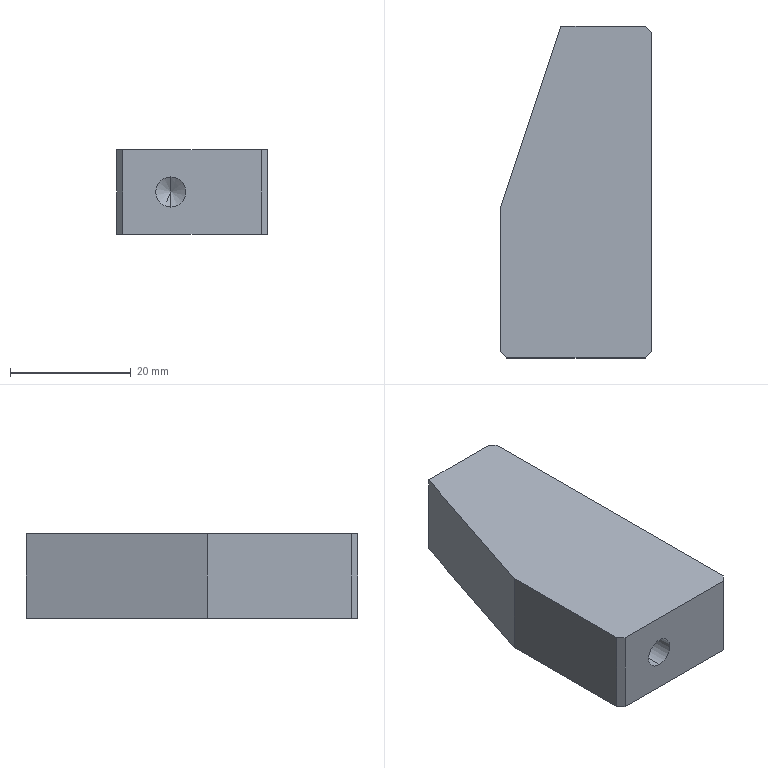Part | SolidWorks | features HoleWzd 2, Chamfer 1, Extrusion 1 | 1 solid | 22 faces | box 25 x 55 x 14 mm | volume 16216 mm3 | plane 10 | cylinder 6 | cone 6 | commonest cylinder face diameters 5 x6
STEP:
#1=CARTESIAN_POINT('',(-16.,15.,2.5));
#2=VERTEX_POINT('',#1);
#3=CARTESIAN_POINT('',(-16.,15.,-2.5));
#4=VERTEX_POINT('',#3);
#5=CARTESIAN_POINT('',(-16.,15.,0.));
#6=DIRECTION('',(0.,-1.,0.));
#7=DIRECTION('',(0.,0.,-1.));
#8=AXIS2_PLACEMENT_3D('',#5,#6,#7);
#9=CIRCLE('',#8,2.5);
#10=EDGE_CURVE('',#2,#4,#9,.T.);
#11=ORIENTED_EDGE('',*,*,#10,.F.);
#12=CARTESIAN_POINT('',(-16.,0.,2.5));
#13=VERTEX_POINT('',#12);
#14=CARTESIAN_POINT('',(-16.,0.,2.5));
#15=DIRECTION('',(0.,-1.,0.));
#16=VECTOR('',#15,1000.);
#17=LINE('',#14,#16);
#18=EDGE_CURVE('',#2,#13,#17,.T.);
#19=ORIENTED_EDGE('',*,*,#18,.T.);
#20=CARTESIAN_POINT('',(-16.,0.,-2.5));
#21=VERTEX_POINT('',#20);
#22=CARTESIAN_POINT('',(-16.,0.,0.));
#23=DIRECTION('',(0.,-1.,0.));
#24=DIRECTION('',(0.,0.,-1.));
#25=AXIS2_PLACEMENT_3D('',#22,#23,#24);
#26=CIRCLE('',#25,2.5);
#27=EDGE_CURVE('',#13,#21,#26,.T.);
#28=ORIENTED_EDGE('',*,*,#27,.T.);
#29=CARTESIAN_POINT('',(-16.,0.,-2.5));
#30=DIRECTION('',(0.,-1.,0.));
#31=VECTOR('',#30,1000.);
#32=LINE('',#29,#31);
#33=EDGE_CURVE('',#4,#21,#32,.T.);
#34=ORIENTED_EDGE('',*,*,#33,.F.);
#35=EDGE_LOOP('',(#11,#19,#28,#34));
#36=FACE_OUTER_BOUND('',#35,.T.);
#37=CARTESIAN_POINT('',(-16.,0.,0.));
#38=DIRECTION('',(0.,-1.,0.));
#39=DIRECTION('',(0.,0.,-1.));
#40=AXIS2_PLACEMENT_3D('',#37,#38,#39);
#41=CYLINDRICAL_SURFACE('',#40,2.5);
#42=ADVANCED_FACE('',(#36),#41,.F.);
#43=CARTESIAN_POINT('',(-16.,16.502,0.));
#44=VERTEX_POINT('',#43);
#45=CARTESIAN_POINT('',(-16.,15.,-2.5));
#46=DIRECTION('',(0.,-0.515,-0.8572));
#47=VECTOR('',#46,1000.);
#48=LINE('',#45,#47);
#49=EDGE_CURVE('',#44,#4,#48,.T.);
#50=ORIENTED_EDGE('',*,*,#49,.F.);
#51=CARTESIAN_POINT('',(-16.,15.,2.5));
#52=DIRECTION('',(0.,-0.515,0.8572));
#53=VECTOR('',#52,1000.);
#54=LINE('',#51,#53);
#55=EDGE_CURVE('',#44,#2,#54,.T.);
#56=ORIENTED_EDGE('',*,*,#55,.T.);
#57=ORIENTED_EDGE('',*,*,#10,.T.);
#58=EDGE_LOOP('',(#50,#56,#57));
#59=FACE_OUTER_BOUND('',#58,.T.);
#60=CARTESIAN_POINT('',(-16.,15.,0.));
#61=DIRECTION('',(0.,-1.,0.));
#62=DIRECTION('',(0.,0.,-1.));
#63=AXIS2_PLACEMENT_3D('',#60,#61,#62);
#64=CONICAL_SURFACE('',#63,2.5,1.03);
#65=ADVANCED_FACE('',(#59),#64,.F.);
#66=CARTESIAN_POINT('',(-15.,47.,2.5));
#67=VERTEX_POINT('',#66);
#68=CARTESIAN_POINT('',(-15.,47.,-2.5));
#69=VERTEX_POINT('',#68);
#70=CARTESIAN_POINT('',(-15.,47.,0.));
#71=DIRECTION('',(1.,0.,0.));
#72=DIRECTION('',(0.,0.,-1.));
#73=AXIS2_PLACEMENT_3D('',#70,#71,#72);
#74=CIRCLE('',#73,2.5);
#75=EDGE_CURVE('',#67,#69,#74,.T.);
#76=ORIENTED_EDGE('',*,*,#75,.F.);
#77=CARTESIAN_POINT('',(0.,47.,2.5));
#78=VERTEX_POINT('',#77);
#79=CARTESIAN_POINT('',(0.,47.,2.5));
#80=DIRECTION('',(1.,0.,0.));
#81=VECTOR('',#80,1000.);
#82=LINE('',#79,#81);
#83=EDGE_CURVE('',#67,#78,#82,.T.);
#84=ORIENTED_EDGE('',*,*,#83,.T.);
#85=CARTESIAN_POINT('',(0.,47.,-2.5));
#86=VERTEX_POINT('',#85);
#87=CARTESIAN_POINT('',(0.,47.,0.));
#88=DIRECTION('',(1.,0.,0.));
#89=DIRECTION('',(0.,0.,-1.));
#90=AXIS2_PLACEMENT_3D('',#87,#88,#89);
#91=CIRCLE('',#90,2.5);
#92=EDGE_CURVE('',#78,#86,#91,.T.);
#93=ORIENTED_EDGE('',*,*,#92,.T.);
#94=CARTESIAN_POINT('',(0.,47.,-2.5));
#95=DIRECTION('',(1.,0.,0.));
#96=VECTOR('',#95,1000.);
#97=LINE('',#94,#96);
#98=EDGE_CURVE('',#69,#86,#97,.T.);
#99=ORIENTED_EDGE('',*,*,#98,.F.);
#100=EDGE_LOOP('',(#76,#84,#93,#99));
#101=FACE_OUTER_BOUND('',#100,.T.);
#102=CARTESIAN_POINT('',(0.,47.,0.));
#103=DIRECTION('',(1.,0.,0.));
#104=DIRECTION('',(0.,0.,-1.));
#105=AXIS2_PLACEMENT_3D('',#102,#103,#104);
#106=CYLINDRICAL_SURFACE('',#105,2.5);
#107=ADVANCED_FACE('',(#101),#106,.F.);
#108=CARTESIAN_POINT('',(-16.502,47.,0.));
#109=VERTEX_POINT('',#108);
#110=CARTESIAN_POINT('',(-15.,47.,-2.5));
#111=DIRECTION('',(0.515,0.,-0.8572));
#112=VECTOR('',#111,1000.);
#113=LINE('',#110,#112);
#114=EDGE_CURVE('',#109,#69,#113,.T.);
#115=ORIENTED_EDGE('',*,*,#114,.F.);
#116=CARTESIAN_POINT('',(-15.,47.,2.5));
#117=DIRECTION('',(0.515,0.,0.8572));
#118=VECTOR('',#117,1000.);
#119=LINE('',#116,#118);
#120=EDGE_CURVE('',#109,#67,#119,.T.);
#121=ORIENTED_EDGE('',*,*,#120,.T.);
#122=ORIENTED_EDGE('',*,*,#75,.T.);
#123=EDGE_LOOP('',(#115,#121,#122));
#124=FACE_OUTER_BOUND('',#123,.T.);
#125=CARTESIAN_POINT('',(-15.,47.,0.));
#126=DIRECTION('',(1.,0.,0.));
#127=DIRECTION('',(0.,0.,-1.));
#128=AXIS2_PLACEMENT_3D('',#125,#126,#127);
#129=CONICAL_SURFACE('',#128,2.5,1.03);
#130=ADVANCED_FACE('',(#124),#129,.F.);
#131=CARTESIAN_POINT('',(-15.,25.,2.5));
#132=VERTEX_POINT('',#131);
#133=CARTESIAN_POINT('',(-15.,25.,-2.5));
#134=VERTEX_POINT('',#133);
#135=CARTESIAN_POINT('',(-15.,25.,0.));
#136=DIRECTION('',(1.,0.,0.));
#137=DIRECTION('',(0.,0.,-1.));
#138=AXIS2_PLACEMENT_3D('',#135,#136,#137);
#139=CIRCLE('',#138,2.5);
#140=EDGE_CURVE('',#132,#134,#139,.T.);
#141=ORIENTED_EDGE('',*,*,#140,.F.);
#142=CARTESIAN_POINT('',(0.,25.,2.5));
#143=VERTEX_POINT('',#142);
#144=CARTESIAN_POINT('',(0.,25.,2.5));
#145=DIRECTION('',(1.,0.,0.));
#146=VECTOR('',#145,1000.);
#147=LINE('',#144,#146);
#148=EDGE_CURVE('',#132,#143,#147,.T.);
#149=ORIENTED_EDGE('',*,*,#148,.T.);
#150=CARTESIAN_POINT('',(0.,25.,-2.5));
#151=VERTEX_POINT('',#150);
#152=CARTESIAN_POINT('',(0.,25.,0.));
#153=DIRECTION('',(1.,0.,0.));
#154=DIRECTION('',(0.,0.,-1.));
#155=AXIS2_PLACEMENT_3D('',#152,#153,#154);
#156=CIRCLE('',#155,2.5);
#157=EDGE_CURVE('',#143,#151,#156,.T.);
#158=ORIENTED_EDGE('',*,*,#157,.T.);
#159=CARTESIAN_POINT('',(0.,25.,-2.5));
#160=DIRECTION('',(1.,0.,0.));
#161=VECTOR('',#160,1000.);
#162=LINE('',#159,#161);
#163=EDGE_CURVE('',#134,#151,#162,.T.);
#164=ORIENTED_EDGE('',*,*,#163,.F.);
#165=EDGE_LOOP('',(#141,#149,#158,#164));
#166=FACE_OUTER_BOUND('',#165,.T.);
#167=CARTESIAN_POINT('',(0.,25.,0.));
#168=DIRECTION('',(1.,0.,0.));
#169=DIRECTION('',(0.,0.,-1.));
#170=AXIS2_PLACEMENT_3D('',#167,#168,#169);
#171=CYLINDRICAL_SURFACE('',#170,2.5);
#172=ADVANCED_FACE('',(#166),#171,.F.);
#173=CARTESIAN_POINT('',(-16.502,25.,0.));
#174=VERTEX_POINT('',#173);
#175=CARTESIAN_POINT('',(-15.,25.,-2.5));
#176=DIRECTION('',(0.515,0.,-0.8572));
#177=VECTOR('',#176,1000.);
#178=LINE('',#175,#177);
#179=EDGE_CURVE('',#174,#134,#178,.T.);
#180=ORIENTED_EDGE('',*,*,#179,.F.);
#181=CARTESIAN_POINT('',(-15.,25.,2.5));
#182=DIRECTION('',(0.515,0.,0.8572));
#183=VECTOR('',#182,1000.);
#184=LINE('',#181,#183);
#185=EDGE_CURVE('',#174,#132,#184,.T.);
#186=ORIENTED_EDGE('',*,*,#185,.T.);
#187=ORIENTED_EDGE('',*,*,#140,.T.);
#188=EDGE_LOOP('',(#180,#186,#187));
#189=FACE_OUTER_BOUND('',#188,.T.);
#190=CARTESIAN_POINT('',(-15.,25.,0.));
#191=DIRECTION('',(1.,0.,0.));
#192=DIRECTION('',(0.,0.,-1.));
#193=AXIS2_PLACEMENT_3D('',#190,#191,#192);
#194=CONICAL_SURFACE('',#193,2.5,1.03);
#195=ADVANCED_FACE('',(#189),#194,.F.);
#196=CARTESIAN_POINT('',(-16.,0.,0.));
#197=DIRECTION('',(0.,-1.,0.));
#198=DIRECTION('',(0.,0.,-1.));
#199=AXIS2_PLACEMENT_3D('',#196,#197,#198);
#200=CIRCLE('',#199,2.5);
#201=EDGE_CURVE('',#21,#13,#200,.T.);
#202=ORIENTED_EDGE('',*,*,#201,.F.);
#203=ORIENTED_EDGE('',*,*,#27,.F.);
#204=EDGE_LOOP('',(#202,#203));
#205=FACE_BOUND('',#204,.T.);
#206=CARTESIAN_POINT('',(-24.,0.,7.));
#207=VERTEX_POINT('',#206);
#208=CARTESIAN_POINT('',(-1.,0.,7.));
#209=VERTEX_POINT('',#208);
#210=CARTESIAN_POINT('',(-25.,0.,7.));
#211=DIRECTION('',(1.,0.,0.));
#212=VECTOR('',#211,1000.);
#213=LINE('',#210,#212);
#214=EDGE_CURVE('',#207,#209,#213,.T.);
#215=ORIENTED_EDGE('',*,*,#214,.F.);
#216=CARTESIAN_POINT('',(-24.,0.,-7.));
#217=VERTEX_POINT('',#216);
#218=CARTESIAN_POINT('',(-24.,0.,7.));
#219=DIRECTION('',(0.,0.,-1.));
#220=VECTOR('',#219,1000.);
#221=LINE('',#218,#220);
#222=EDGE_CURVE('',#207,#217,#221,.T.);
#223=ORIENTED_EDGE('',*,*,#222,.T.);
#224=CARTESIAN_POINT('',(-1.,0.,-7.));
#225=VERTEX_POINT('',#224);
#226=CARTESIAN_POINT('',(-25.,0.,-7.));
#227=DIRECTION('',(1.,0.,0.));
#228=VECTOR('',#227,1000.);
#229=LINE('',#226,#228);
#230=EDGE_CURVE('',#217,#225,#229,.T.);
#231=ORIENTED_EDGE('',*,*,#230,.T.);
#232=CARTESIAN_POINT('',(-1.,0.,7.));
#233=DIRECTION('',(0.,0.,1.));
#234=VECTOR('',#233,1000.);
#235=LINE('',#232,#234);
#236=EDGE_CURVE('',#225,#209,#235,.T.);
#237=ORIENTED_EDGE('',*,*,#236,.T.);
#238=EDGE_LOOP('',(#215,#223,#231,#237));
#239=FACE_OUTER_BOUND('',#238,.T.);
#240=CARTESIAN_POINT('',(-25.,0.,7.));
#241=DIRECTION('',(0.,1.,0.));
#242=DIRECTION('',(0.,0.,1.));
#243=AXIS2_PLACEMENT_3D('',#240,#241,#242);
#244=PLANE('',#243);
#245=ADVANCED_FACE('',(#205,#239),#244,.F.);
#246=CARTESIAN_POINT('',(0.,47.,0.));
#247=DIRECTION('',(1.,0.,0.));
#248=DIRECTION('',(0.,0.,-1.));
#249=AXIS2_PLACEMENT_3D('',#246,#247,#248);
#250=CIRCLE('',#249,2.5);
#251=EDGE_CURVE('',#86,#78,#250,.T.);
#252=ORIENTED_EDGE('',*,*,#251,.F.);
#253=ORIENTED_EDGE('',*,*,#92,.F.);
#254=EDGE_LOOP('',(#252,#253));
#255=FACE_BOUND('',#254,.T.);
#256=CARTESIAN_POINT('',(0.,25.,0.));
#257=DIRECTION('',(1.,0.,0.));
#258=DIRECTION('',(0.,0.,-1.));
#259=AXIS2_PLACEMENT_3D('',#256,#257,#258);
#260=CIRCLE('',#259,2.5);
#261=EDGE_CURVE('',#151,#143,#260,.T.);
#262=ORIENTED_EDGE('',*,*,#261,.F.);
#263=ORIENTED_EDGE('',*,*,#157,.F.);
#264=EDGE_LOOP('',(#262,#263));
#265=FACE_BOUND('',#264,.T.);
#266=CARTESIAN_POINT('',(0.,1.,7.));
#267=VERTEX_POINT('',#266);
#268=CARTESIAN_POINT('',(0.,54.,7.));
#269=VERTEX_POINT('',#268);
#270=CARTESIAN_POINT('',(0.,0.,7.));
#271=DIRECTION('',(0.,1.,0.));
#272=VECTOR('',#271,1000.);
#273=LINE('',#270,#272);
#274=EDGE_CURVE('',#267,#269,#273,.T.);
#275=ORIENTED_EDGE('',*,*,#274,.F.);
#276=CARTESIAN_POINT('',(0.,1.,-7.));
#277=VERTEX_POINT('',#276);
#278=CARTESIAN_POINT('',(0.,1.,7.));
#279=DIRECTION('',(0.,0.,-1.));
#280=VECTOR('',#279,1000.);
#281=LINE('',#278,#280);
#282=EDGE_CURVE('',#267,#277,#281,.T.);
#283=ORIENTED_EDGE('',*,*,#282,.T.);
#284=CARTESIAN_POINT('',(0.,54.,-7.));
#285=VERTEX_POINT('',#284);
#286=CARTESIAN_POINT('',(0.,0.,-7.));
#287=DIRECTION('',(0.,1.,0.));
#288=VECTOR('',#287,1000.);
#289=LINE('',#286,#288);
#290=EDGE_CURVE('',#277,#285,#289,.T.);
#291=ORIENTED_EDGE('',*,*,#290,.T.);
#292=CARTESIAN_POINT('',(0.,54.,7.));
#293=DIRECTION('',(0.,0.,1.));
#294=VECTOR('',#293,1000.);
#295=LINE('',#292,#294);
#296=EDGE_CURVE('',#285,#269,#295,.T.);
#297=ORIENTED_EDGE('',*,*,#296,.T.);
#298=EDGE_LOOP('',(#275,#283,#291,#297));
#299=FACE_OUTER_BOUND('',#298,.T.);
#300=CARTESIAN_POINT('',(0.,0.,7.));
#301=DIRECTION('',(-1.,0.,0.));
#302=DIRECTION('',(0.,0.,1.));
#303=AXIS2_PLACEMENT_3D('',#300,#301,#302);
#304=PLANE('',#303);
#305=ADVANCED_FACE('',(#255,#265,#299),#304,.F.);
#306=CARTESIAN_POINT('',(-1.,55.,7.));
#307=VERTEX_POINT('',#306);
#308=CARTESIAN_POINT('',(-15.,55.,7.));
#309=VERTEX_POINT('',#308);
#310=CARTESIAN_POINT('',(0.,55.,7.));
#311=DIRECTION('',(-1.,0.,0.));
#312=VECTOR('',#311,1000.);
#313=LINE('',#310,#312);
#314=EDGE_CURVE('',#307,#309,#313,.T.);
#315=ORIENTED_EDGE('',*,*,#314,.F.);
#316=CARTESIAN_POINT('',(-1.,55.,-7.));
#317=VERTEX_POINT('',#316);
#318=CARTESIAN_POINT('',(-1.,55.,7.));
#319=DIRECTION('',(0.,0.,-1.));
#320=VECTOR('',#319,1000.);
#321=LINE('',#318,#320);
#322=EDGE_CURVE('',#307,#317,#321,.T.);
#323=ORIENTED_EDGE('',*,*,#322,.T.);
#324=CARTESIAN_POINT('',(-15.,55.,-7.));
#325=VERTEX_POINT('',#324);
#326=CARTESIAN_POINT('',(0.,55.,-7.));
#327=DIRECTION('',(-1.,0.,0.));
#328=VECTOR('',#327,1000.);
#329=LINE('',#326,#328);
#330=EDGE_CURVE('',#317,#325,#329,.T.);
#331=ORIENTED_EDGE('',*,*,#330,.T.);
#332=CARTESIAN_POINT('',(-15.,55.,7.));
#333=DIRECTION('',(0.,0.,-1.));
#334=VECTOR('',#333,1000.);
#335=LINE('',#332,#334);
#336=EDGE_CURVE('',#309,#325,#335,.T.);
#337=ORIENTED_EDGE('',*,*,#336,.F.);
#338=EDGE_LOOP('',(#315,#323,#331,#337));
#339=FACE_OUTER_BOUND('',#338,.T.);
#340=CARTESIAN_POINT('',(0.,55.,7.));
#341=DIRECTION('',(0.,-1.,0.));
#342=DIRECTION('',(0.,0.,-1.));
#343=AXIS2_PLACEMENT_3D('',#340,#341,#342);
#344=PLANE('',#343);
#345=ADVANCED_FACE('',(#339),#344,.F.);
#346=CARTESIAN_POINT('',(-25.,25.,-7.));
#347=VERTEX_POINT('',#346);
#348=CARTESIAN_POINT('',(-25.,25.,-7.));
#349=DIRECTION('',(-0.3162,-0.9487,0.));
#350=VECTOR('',#349,1000.);
#351=LINE('',#348,#350);
#352=EDGE_CURVE('',#325,#347,#351,.T.);
#353=ORIENTED_EDGE('',*,*,#352,.T.);
#354=CARTESIAN_POINT('',(-25.,25.,7.));
#355=VERTEX_POINT('',#354);
#356=CARTESIAN_POINT('',(-25.,25.,7.));
#357=DIRECTION('',(0.,0.,-1.));
#358=VECTOR('',#357,1000.);
#359=LINE('',#356,#358);
#360=EDGE_CURVE('',#355,#347,#359,.T.);
#361=ORIENTED_EDGE('',*,*,#360,.F.);
#362=CARTESIAN_POINT('',(-25.,25.,7.));
#363=DIRECTION('',(-0.3162,-0.9487,0.));
#364=VECTOR('',#363,1000.);
#365=LINE('',#362,#364);
#366=EDGE_CURVE('',#309,#355,#365,.T.);
#367=ORIENTED_EDGE('',*,*,#366,.F.);
#368=ORIENTED_EDGE('',*,*,#336,.T.);
#369=EDGE_LOOP('',(#353,#361,#367,#368));
#370=FACE_OUTER_BOUND('',#369,.T.);
#371=CARTESIAN_POINT('',(-25.,25.,7.));
#372=DIRECTION('',(0.9487,-0.3162,0.));
#373=DIRECTION('',(0.3162,0.9487,0.));
#374=AXIS2_PLACEMENT_3D('',#371,#372,#373);
#375=PLANE('',#374);
#376=ADVANCED_FACE('',(#370),#375,.F.);
#377=CARTESIAN_POINT('',(-25.,1.,-7.));
#378=VERTEX_POINT('',#377);
#379=CARTESIAN_POINT('',(-25.,25.,-7.));
#380=DIRECTION('',(0.,-1.,0.));
#381=VECTOR('',#380,1000.);
#382=LINE('',#379,#381);
#383=EDGE_CURVE('',#347,#378,#382,.T.);
#384=ORIENTED_EDGE('',*,*,#383,.T.);
#385=CARTESIAN_POINT('',(-25.,1.,7.));
#386=VERTEX_POINT('',#385);
#387=CARTESIAN_POINT('',(-25.,1.,7.));
#388=DIRECTION('',(0.,0.,1.));
#389=VECTOR('',#388,1000.);
#390=LINE('',#387,#389);
#391=EDGE_CURVE('',#378,#386,#390,.T.);
#392=ORIENTED_EDGE('',*,*,#391,.T.);
#393=CARTESIAN_POINT('',(-25.,25.,7.));
#394=DIRECTION('',(0.,-1.,0.));
#395=VECTOR('',#394,1000.);
#396=LINE('',#393,#395);
#397=EDGE_CURVE('',#355,#386,#396,.T.);
#398=ORIENTED_EDGE('',*,*,#397,.F.);
#399=ORIENTED_EDGE('',*,*,#360,.T.);
#400=EDGE_LOOP('',(#384,#392,#398,#399));
#401=FACE_OUTER_BOUND('',#400,.T.);
#402=CARTESIAN_POINT('',(-25.,25.,7.));
#403=DIRECTION('',(1.,0.,0.));
#404=DIRECTION('',(0.,0.,-1.));
#405=AXIS2_PLACEMENT_3D('',#402,#403,#404);
#406=PLANE('',#405);
#407=ADVANCED_FACE('',(#401),#406,.F.);
#408=ORIENTED_EDGE('',*,*,#397,.T.);
#409=CARTESIAN_POINT('',(-12.,-12.,7.));
#410=DIRECTION('',(0.7071,-0.7071,0.));
#411=VECTOR('',#410,1000.);
#412=LINE('',#409,#411);
#413=EDGE_CURVE('',#386,#207,#412,.T.);
#414=ORIENTED_EDGE('',*,*,#413,.T.);
#415=ORIENTED_EDGE('',*,*,#214,.T.);
#416=CARTESIAN_POINT('',(-0.5,0.5,7.));
#417=DIRECTION('',(0.7071,0.7071,0.));
#418=VECTOR('',#417,1000.);
#419=LINE('',#416,#418);
#420=EDGE_CURVE('',#209,#267,#419,.T.);
#421=ORIENTED_EDGE('',*,*,#420,.T.);
#422=ORIENTED_EDGE('',*,*,#274,.T.);
#423=CARTESIAN_POINT('',(27.,27.,7.));
#424=DIRECTION('',(-0.7071,0.7071,0.));
#425=VECTOR('',#424,1000.);
#426=LINE('',#423,#425);
#427=EDGE_CURVE('',#269,#307,#426,.T.);
#428=ORIENTED_EDGE('',*,*,#427,.T.);
#429=ORIENTED_EDGE('',*,*,#314,.T.);
#430=ORIENTED_EDGE('',*,*,#366,.T.);
#431=EDGE_LOOP('',(#408,#414,#415,#421,#422,#428,#429,#430));
#432=FACE_OUTER_BOUND('',#431,.T.);
#433=CARTESIAN_POINT('',(0.,0.,7.));
#434=DIRECTION('',(0.,0.,1.));
#435=DIRECTION('',(1.,0.,0.));
#436=AXIS2_PLACEMENT_3D('',#433,#434,#435);
#437=PLANE('',#436);
#438=ADVANCED_FACE('',(#432),#437,.T.);
#439=ORIENTED_EDGE('',*,*,#230,.F.);
#440=CARTESIAN_POINT('',(-24.,0.,-7.));
#441=DIRECTION('',(-0.7071,0.7071,0.));
#442=VECTOR('',#441,1000.);
#443=LINE('',#440,#442);
#444=EDGE_CURVE('',#217,#378,#443,.T.);
#445=ORIENTED_EDGE('',*,*,#444,.T.);
#446=ORIENTED_EDGE('',*,*,#383,.F.);
#447=ORIENTED_EDGE('',*,*,#352,.F.);
#448=ORIENTED_EDGE('',*,*,#330,.F.);
#449=CARTESIAN_POINT('',(-1.,55.,-7.));
#450=DIRECTION('',(0.7071,-0.7071,0.));
#451=VECTOR('',#450,1000.);
#452=LINE('',#449,#451);
#453=EDGE_CURVE('',#317,#285,#452,.T.);
#454=ORIENTED_EDGE('',*,*,#453,.T.);
#455=ORIENTED_EDGE('',*,*,#290,.F.);
#456=CARTESIAN_POINT('',(0.,1.,-7.));
#457=DIRECTION('',(-0.7071,-0.7071,0.));
#458=VECTOR('',#457,1000.);
#459=LINE('',#456,#458);
#460=EDGE_CURVE('',#277,#225,#459,.T.);
#461=ORIENTED_EDGE('',*,*,#460,.T.);
#462=EDGE_LOOP('',(#439,#445,#446,#447,#448,#454,#455,#461));
#463=FACE_OUTER_BOUND('',#462,.T.);
#464=CARTESIAN_POINT('',(0.,0.,-7.));
#465=DIRECTION('',(0.,0.,1.));
#466=DIRECTION('',(1.,0.,0.));
#467=AXIS2_PLACEMENT_3D('',#464,#465,#466);
#468=PLANE('',#467);
#469=ADVANCED_FACE('',(#463),#468,.F.);
#470=ORIENTED_EDGE('',*,*,#185,.F.);
#471=ORIENTED_EDGE('',*,*,#179,.T.);
#472=CARTESIAN_POINT('',(-15.,25.,0.));
#473=DIRECTION('',(1.,0.,0.));
#474=DIRECTION('',(0.,0.,-1.));
#475=AXIS2_PLACEMENT_3D('',#472,#473,#474);
#476=CIRCLE('',#475,2.5);
#477=EDGE_CURVE('',#134,#132,#476,.T.);
#478=ORIENTED_EDGE('',*,*,#477,.T.);
#479=EDGE_LOOP('',(#470,#471,#478));
#480=FACE_OUTER_BOUND('',#479,.T.);
#481=CARTESIAN_POINT('',(-15.,25.,0.));
#482=DIRECTION('',(1.,0.,0.));
#483=DIRECTION('',(0.,0.,-1.));
#484=AXIS2_PLACEMENT_3D('',#481,#482,#483);
#485=CONICAL_SURFACE('',#484,2.5,1.03);
#486=ADVANCED_FACE('',(#480),#485,.F.);
#487=ORIENTED_EDGE('',*,*,#148,.F.);
#488=ORIENTED_EDGE('',*,*,#477,.F.);
#489=ORIENTED_EDGE('',*,*,#163,.T.);
#490=ORIENTED_EDGE('',*,*,#261,.T.);
#491=EDGE_LOOP('',(#487,#488,#489,#490));
#492=FACE_OUTER_BOUND('',#491,.T.);
#493=CARTESIAN_POINT('',(0.,25.,0.));
#494=DIRECTION('',(1.,0.,0.));
#495=DIRECTION('',(0.,0.,-1.));
#496=AXIS2_PLACEMENT_3D('',#493,#494,#495);
#497=CYLINDRICAL_SURFACE('',#496,2.5);
#498=ADVANCED_FACE('',(#492),#497,.F.);
#499=ORIENTED_EDGE('',*,*,#120,.F.);
#500=ORIENTED_EDGE('',*,*,#114,.T.);
#501=CARTESIAN_POINT('',(-15.,47.,0.));
#502=DIRECTION('',(1.,0.,0.));
#503=DIRECTION('',(0.,0.,-1.));
#504=AXIS2_PLACEMENT_3D('',#501,#502,#503);
#505=CIRCLE('',#504,2.5);
#506=EDGE_CURVE('',#69,#67,#505,.T.);
#507=ORIENTED_EDGE('',*,*,#506,.T.);
#508=EDGE_LOOP('',(#499,#500,#507));
#509=FACE_OUTER_BOUND('',#508,.T.);
#510=CARTESIAN_POINT('',(-15.,47.,0.));
#511=DIRECTION('',(1.,0.,0.));
#512=DIRECTION('',(0.,0.,-1.));
#513=AXIS2_PLACEMENT_3D('',#510,#511,#512);
#514=CONICAL_SURFACE('',#513,2.5,1.03);
#515=ADVANCED_FACE('',(#509),#514,.F.);
#516=ORIENTED_EDGE('',*,*,#83,.F.);
#517=ORIENTED_EDGE('',*,*,#506,.F.);
#518=ORIENTED_EDGE('',*,*,#98,.T.);
#519=ORIENTED_EDGE('',*,*,#251,.T.);
#520=EDGE_LOOP('',(#516,#517,#518,#519));
#521=FACE_OUTER_BOUND('',#520,.T.);
#522=CARTESIAN_POINT('',(0.,47.,0.));
#523=DIRECTION('',(1.,0.,0.));
#524=DIRECTION('',(0.,0.,-1.));
#525=AXIS2_PLACEMENT_3D('',#522,#523,#524);
#526=CYLINDRICAL_SURFACE('',#525,2.5);
#527=ADVANCED_FACE('',(#521),#526,.F.);
#528=ORIENTED_EDGE('',*,*,#55,.F.);
#529=ORIENTED_EDGE('',*,*,#49,.T.);
#530=CARTESIAN_POINT('',(-16.,15.,0.));
#531=DIRECTION('',(0.,-1.,0.));
#532=DIRECTION('',(0.,0.,-1.));
#533=AXIS2_PLACEMENT_3D('',#530,#531,#532);
#534=CIRCLE('',#533,2.5);
#535=EDGE_CURVE('',#4,#2,#534,.T.);
#536=ORIENTED_EDGE('',*,*,#535,.T.);
#537=EDGE_LOOP('',(#528,#529,#536));
#538=FACE_OUTER_BOUND('',#537,.T.);
#539=CARTESIAN_POINT('',(-16.,15.,0.));
#540=DIRECTION('',(0.,-1.,0.));
#541=DIRECTION('',(0.,0.,-1.));
#542=AXIS2_PLACEMENT_3D('',#539,#540,#541);
#543=CONICAL_SURFACE('',#542,2.5,1.03);
#544=ADVANCED_FACE('',(#538),#543,.F.);
#545=ORIENTED_EDGE('',*,*,#18,.F.);
#546=ORIENTED_EDGE('',*,*,#535,.F.);
#547=ORIENTED_EDGE('',*,*,#33,.T.);
#548=ORIENTED_EDGE('',*,*,#201,.T.);
#549=EDGE_LOOP('',(#545,#546,#547,#548));
#550=FACE_OUTER_BOUND('',#549,.T.);
#551=CARTESIAN_POINT('',(-16.,0.,0.));
#552=DIRECTION('',(0.,-1.,0.));
#553=DIRECTION('',(0.,0.,-1.));
#554=AXIS2_PLACEMENT_3D('',#551,#552,#553);
#555=CYLINDRICAL_SURFACE('',#554,2.5);
#556=ADVANCED_FACE('',(#550),#555,.F.);
#557=ORIENTED_EDGE('',*,*,#413,.F.);
#558=ORIENTED_EDGE('',*,*,#391,.F.);
#559=ORIENTED_EDGE('',*,*,#444,.F.);
#560=ORIENTED_EDGE('',*,*,#222,.F.);
#561=EDGE_LOOP('',(#557,#558,#559,#560));
#562=FACE_OUTER_BOUND('',#561,.T.);
#563=CARTESIAN_POINT('',(-24.,0.,7.));
#564=DIRECTION('',(0.7071,0.7071,0.));
#565=DIRECTION('',(0.,0.,-1.));
#566=AXIS2_PLACEMENT_3D('',#563,#564,#565);
#567=PLANE('',#566);
#568=ADVANCED_FACE('',(#562),#567,.F.);
#569=ORIENTED_EDGE('',*,*,#420,.F.);
#570=ORIENTED_EDGE('',*,*,#236,.F.);
#571=ORIENTED_EDGE('',*,*,#460,.F.);
#572=ORIENTED_EDGE('',*,*,#282,.F.);
#573=EDGE_LOOP('',(#569,#570,#571,#572));
#574=FACE_OUTER_BOUND('',#573,.T.);
#575=CARTESIAN_POINT('',(0.,1.,7.));
#576=DIRECTION('',(-0.7071,0.7071,0.));
#577=DIRECTION('',(0.,0.,-1.));
#578=AXIS2_PLACEMENT_3D('',#575,#576,#577);
#579=PLANE('',#578);
#580=ADVANCED_FACE('',(#574),#579,.F.);
#581=ORIENTED_EDGE('',*,*,#427,.F.);
#582=ORIENTED_EDGE('',*,*,#296,.F.);
#583=ORIENTED_EDGE('',*,*,#453,.F.);
#584=ORIENTED_EDGE('',*,*,#322,.F.);
#585=EDGE_LOOP('',(#581,#582,#583,#584));
#586=FACE_OUTER_BOUND('',#585,.T.);
#587=CARTESIAN_POINT('',(-1.,55.,7.));
#588=DIRECTION('',(-0.7071,-0.7071,0.));
#589=DIRECTION('',(0.,0.,-1.));
#590=AXIS2_PLACEMENT_3D('',#587,#588,#589);
#591=PLANE('',#590);
#592=ADVANCED_FACE('',(#586),#591,.F.);
#593=CLOSED_SHELL('',(#42,#65,#107,#130,#172,#195,#245,#305,#345,#376,#407,#438,#469,#486,#498,#515,#527,#544,#556,#568,#580,#592));
#594=MANIFOLD_SOLID_BREP('',#593);
#595=CARTESIAN_POINT('',(0.,0.,0.));
#596=DIRECTION('',(0.,0.,1.));
#597=DIRECTION('',(1.,0.,0.));
#598=AXIS2_PLACEMENT_3D('',#595,#596,#597);
#599=(LENGTH_UNIT()NAMED_UNIT(*)SI_UNIT(.MILLI.,.METRE.));
#600=UNCERTAINTY_MEASURE_WITH_UNIT(LENGTH_MEASURE(0.00001),#599,'','');
#601=(NAMED_UNIT(*)PLANE_ANGLE_UNIT()SI_UNIT($,.RADIAN.));
#602=(NAMED_UNIT(*)SI_UNIT($,.STERADIAN.)SOLID_ANGLE_UNIT());
#603=(GEOMETRIC_REPRESENTATION_CONTEXT(3)GLOBAL_UNCERTAINTY_ASSIGNED_CONTEXT((#600))GLOBAL_UNIT_ASSIGNED_CONTEXT((#599,#601,#602))REPRESENTATION_CONTEXT('',''));
#604=ADVANCED_BREP_SHAPE_REPRESENTATION('',(#594,#598),#603);